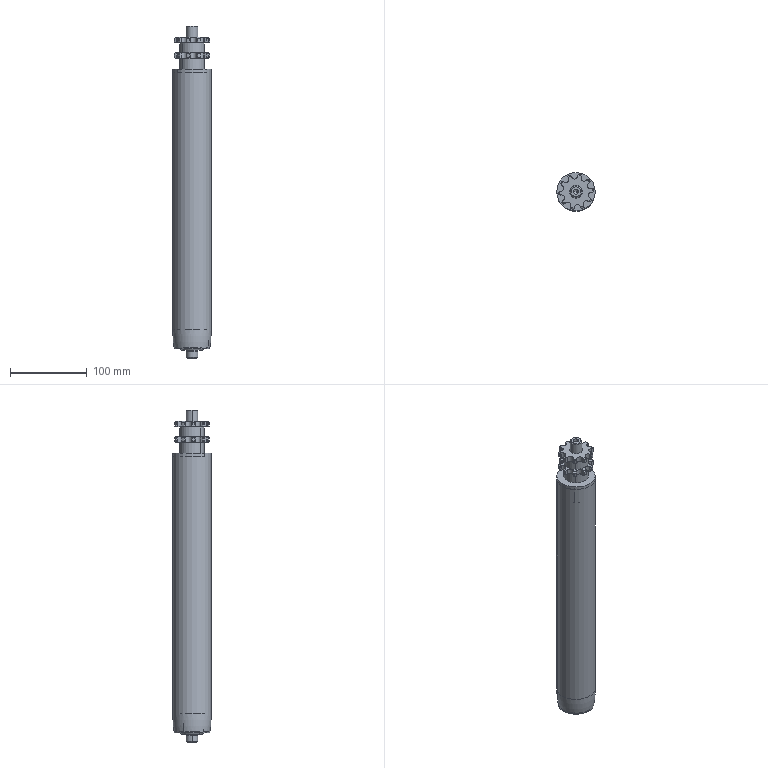Part | SolidWorks | 4 solids | 239 faces | box 50 x 50 x 432 mm | volume 219303 mm3 | plane 97 | cylinder 74 | cone 52 | torus 16 | commonest cylinder face diameters 46 x22 7.92 x20 6.8 x4 15 x4 32 x4 47.6 x4